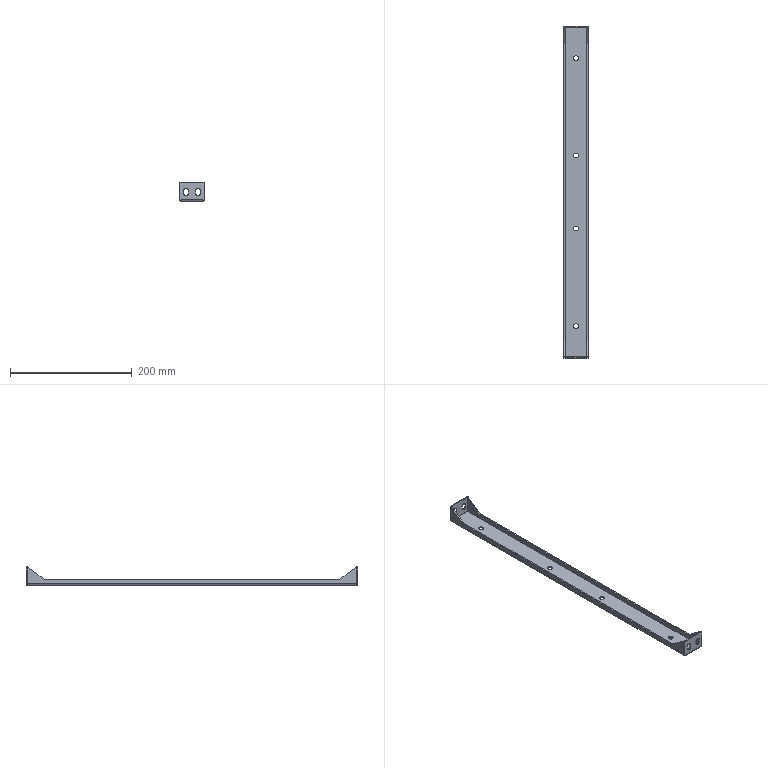Part | SolidWorks | features ICE 3, EdgeFlange 2, FlatPattern 1, SMBaseFlange 1, SheetMetal 1 | 1 solid | 74 faces | box 40 x 545 x 30 mm | volume 65298 mm3 | plane 46 | cylinder 28 | commonest cylinder face diameters 8 x20 0.4 x4 4.4 x4